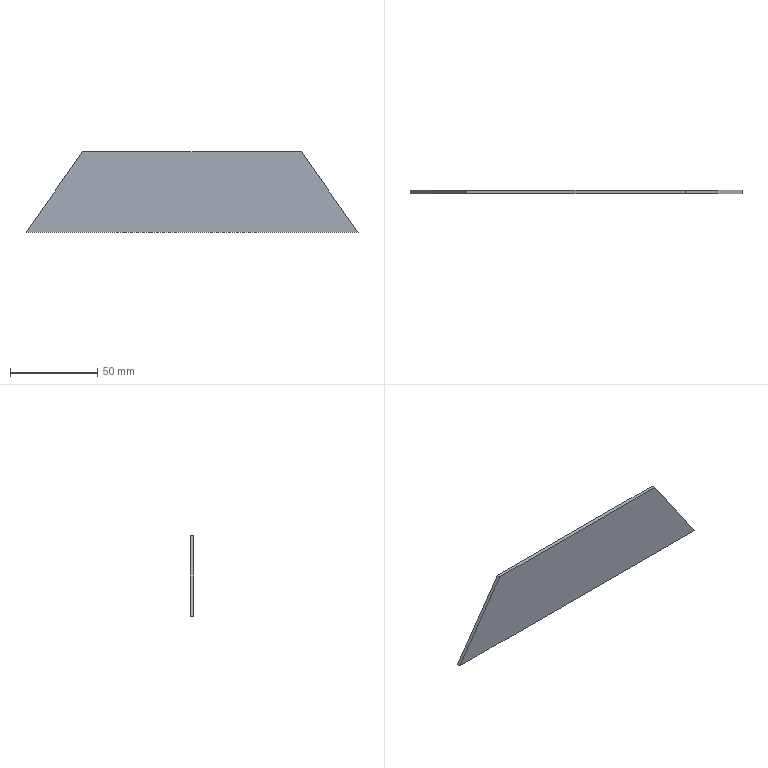Part | SolidWorks | features BaseBody 1 | 1 solid | 6 faces | box 189.769 x 2 x 46.25 mm | volume 14558 mm3 | plane 6
STEP:
#1=CARTESIAN_POINT('',(-157.385,2.,-46.25));
#2=VERTEX_POINT('',#1);
#3=CARTESIAN_POINT('',(-125.,2.,0.));
#4=VERTEX_POINT('',#3);
#5=CARTESIAN_POINT('',(-125.,2.,0.));
#6=DIRECTION('',(0.5736,0.,0.8192));
#7=VECTOR('',#6,1000.);
#8=LINE('',#5,#7);
#9=EDGE_CURVE('',#2,#4,#8,.T.);
#10=ORIENTED_EDGE('',*,*,#9,.T.);
#11=CARTESIAN_POINT('',(0.,2.,0.));
#12=VERTEX_POINT('',#11);
#13=CARTESIAN_POINT('',(0.,2.,0.));
#14=DIRECTION('',(1.,0.,0.));
#15=VECTOR('',#14,1000.);
#16=LINE('',#13,#15);
#17=EDGE_CURVE('',#4,#12,#16,.T.);
#18=ORIENTED_EDGE('',*,*,#17,.T.);
#19=CARTESIAN_POINT('',(32.385,2.,-46.25));
#20=VERTEX_POINT('',#19);
#21=CARTESIAN_POINT('',(0.,2.,0.));
#22=DIRECTION('',(0.5736,0.,-0.8192));
#23=VECTOR('',#22,1000.);
#24=LINE('',#21,#23);
#25=EDGE_CURVE('',#12,#20,#24,.T.);
#26=ORIENTED_EDGE('',*,*,#25,.T.);
#27=CARTESIAN_POINT('',(32.385,2.,-46.25));
#28=DIRECTION('',(-1.,0.,0.));
#29=VECTOR('',#28,1000.);
#30=LINE('',#27,#29);
#31=EDGE_CURVE('',#20,#2,#30,.T.);
#32=ORIENTED_EDGE('',*,*,#31,.T.);
#33=EDGE_LOOP('',(#10,#18,#26,#32));
#34=FACE_OUTER_BOUND('',#33,.T.);
#35=CARTESIAN_POINT('',(0.,2.,0.));
#36=DIRECTION('',(0.,1.,0.));
#37=DIRECTION('',(1.,0.,0.));
#38=AXIS2_PLACEMENT_3D('',#35,#36,#37);
#39=PLANE('',#38);
#40=ADVANCED_FACE('',(#34),#39,.T.);
#41=CARTESIAN_POINT('',(-157.385,0.,-46.25));
#42=VERTEX_POINT('',#41);
#43=CARTESIAN_POINT('',(-157.385,2.,-46.25));
#44=DIRECTION('',(0.,1.,0.));
#45=VECTOR('',#44,1000.);
#46=LINE('',#43,#45);
#47=EDGE_CURVE('',#42,#2,#46,.T.);
#48=ORIENTED_EDGE('',*,*,#47,.T.);
#49=ORIENTED_EDGE('',*,*,#31,.F.);
#50=CARTESIAN_POINT('',(32.385,0.,-46.25));
#51=VERTEX_POINT('',#50);
#52=CARTESIAN_POINT('',(32.385,2.,-46.25));
#53=DIRECTION('',(0.,-1.,0.));
#54=VECTOR('',#53,1000.);
#55=LINE('',#52,#54);
#56=EDGE_CURVE('',#20,#51,#55,.T.);
#57=ORIENTED_EDGE('',*,*,#56,.T.);
#58=CARTESIAN_POINT('',(0.,0.,-46.25));
#59=DIRECTION('',(-1.,0.,0.));
#60=VECTOR('',#59,1000.);
#61=LINE('',#58,#60);
#62=EDGE_CURVE('',#51,#42,#61,.T.);
#63=ORIENTED_EDGE('',*,*,#62,.T.);
#64=EDGE_LOOP('',(#48,#49,#57,#63));
#65=FACE_OUTER_BOUND('',#64,.T.);
#66=CARTESIAN_POINT('',(32.385,2.,-46.25));
#67=DIRECTION('',(0.,0.,1.));
#68=DIRECTION('',(1.,0.,0.));
#69=AXIS2_PLACEMENT_3D('',#66,#67,#68);
#70=PLANE('',#69);
#71=ADVANCED_FACE('',(#65),#70,.F.);
#72=CARTESIAN_POINT('',(-125.,0.,0.));
#73=VERTEX_POINT('',#72);
#74=CARTESIAN_POINT('',(-125.,2.,0.));
#75=DIRECTION('',(0.,1.,0.));
#76=VECTOR('',#75,1000.);
#77=LINE('',#74,#76);
#78=EDGE_CURVE('',#73,#4,#77,.T.);
#79=ORIENTED_EDGE('',*,*,#78,.T.);
#80=ORIENTED_EDGE('',*,*,#9,.F.);
#81=ORIENTED_EDGE('',*,*,#47,.F.);
#82=CARTESIAN_POINT('',(-157.385,0.,-46.25));
#83=DIRECTION('',(0.5736,0.,0.8192));
#84=VECTOR('',#83,1000.);
#85=LINE('',#82,#84);
#86=EDGE_CURVE('',#42,#73,#85,.T.);
#87=ORIENTED_EDGE('',*,*,#86,.T.);
#88=EDGE_LOOP('',(#79,#80,#81,#87));
#89=FACE_OUTER_BOUND('',#88,.T.);
#90=CARTESIAN_POINT('',(-125.,2.,0.));
#91=DIRECTION('',(0.8192,0.,-0.5736));
#92=DIRECTION('',(0.,-1.,0.));
#93=AXIS2_PLACEMENT_3D('',#90,#91,#92);
#94=PLANE('',#93);
#95=ADVANCED_FACE('',(#89),#94,.F.);
#96=CARTESIAN_POINT('',(0.,0.,0.));
#97=VERTEX_POINT('',#96);
#98=CARTESIAN_POINT('',(0.,2.,0.));
#99=DIRECTION('',(0.,1.,0.));
#100=VECTOR('',#99,1000.);
#101=LINE('',#98,#100);
#102=EDGE_CURVE('',#97,#12,#101,.T.);
#103=ORIENTED_EDGE('',*,*,#102,.T.);
#104=ORIENTED_EDGE('',*,*,#17,.F.);
#105=ORIENTED_EDGE('',*,*,#78,.F.);
#106=CARTESIAN_POINT('',(0.,0.,0.));
#107=DIRECTION('',(1.,0.,0.));
#108=VECTOR('',#107,1000.);
#109=LINE('',#106,#108);
#110=EDGE_CURVE('',#73,#97,#109,.T.);
#111=ORIENTED_EDGE('',*,*,#110,.T.);
#112=EDGE_LOOP('',(#103,#104,#105,#111));
#113=FACE_OUTER_BOUND('',#112,.T.);
#114=CARTESIAN_POINT('',(0.,2.,0.));
#115=DIRECTION('',(0.,0.,-1.));
#116=DIRECTION('',(-1.,0.,0.));
#117=AXIS2_PLACEMENT_3D('',#114,#115,#116);
#118=PLANE('',#117);
#119=ADVANCED_FACE('',(#113),#118,.F.);
#120=ORIENTED_EDGE('',*,*,#56,.F.);
#121=ORIENTED_EDGE('',*,*,#25,.F.);
#122=ORIENTED_EDGE('',*,*,#102,.F.);
#123=CARTESIAN_POINT('',(0.,0.,0.));
#124=DIRECTION('',(0.5736,0.,-0.8192));
#125=VECTOR('',#124,1000.);
#126=LINE('',#123,#125);
#127=EDGE_CURVE('',#97,#51,#126,.T.);
#128=ORIENTED_EDGE('',*,*,#127,.T.);
#129=EDGE_LOOP('',(#120,#121,#122,#128));
#130=FACE_OUTER_BOUND('',#129,.T.);
#131=CARTESIAN_POINT('',(0.,2.,0.));
#132=DIRECTION('',(-0.8192,0.,-0.5736));
#133=DIRECTION('',(-0.5736,0.,0.8192));
#134=AXIS2_PLACEMENT_3D('',#131,#132,#133);
#135=PLANE('',#134);
#136=ADVANCED_FACE('',(#130),#135,.F.);
#137=ORIENTED_EDGE('',*,*,#110,.F.);
#138=ORIENTED_EDGE('',*,*,#86,.F.);
#139=ORIENTED_EDGE('',*,*,#62,.F.);
#140=ORIENTED_EDGE('',*,*,#127,.F.);
#141=EDGE_LOOP('',(#137,#138,#139,#140));
#142=FACE_OUTER_BOUND('',#141,.T.);
#143=CARTESIAN_POINT('',(0.,0.,0.));
#144=DIRECTION('',(0.,1.,0.));
#145=DIRECTION('',(1.,0.,0.));
#146=AXIS2_PLACEMENT_3D('',#143,#144,#145);
#147=PLANE('',#146);
#148=ADVANCED_FACE('',(#142),#147,.F.);
#149=CLOSED_SHELL('',(#40,#71,#95,#119,#136,#148));
#150=MANIFOLD_SOLID_BREP('',#149);
#151=CARTESIAN_POINT('',(0.,0.,0.));
#152=DIRECTION('',(0.,0.,1.));
#153=DIRECTION('',(1.,0.,0.));
#154=AXIS2_PLACEMENT_3D('',#151,#152,#153);
#155=(LENGTH_UNIT()NAMED_UNIT(*)SI_UNIT(.MILLI.,.METRE.));
#156=UNCERTAINTY_MEASURE_WITH_UNIT(LENGTH_MEASURE(0.00001),#155,'','');
#157=(NAMED_UNIT(*)PLANE_ANGLE_UNIT()SI_UNIT($,.RADIAN.));
#158=(NAMED_UNIT(*)SI_UNIT($,.STERADIAN.)SOLID_ANGLE_UNIT());
#159=(GEOMETRIC_REPRESENTATION_CONTEXT(3)GLOBAL_UNCERTAINTY_ASSIGNED_CONTEXT((#156))GLOBAL_UNIT_ASSIGNED_CONTEXT((#155,#157,#158))REPRESENTATION_CONTEXT('',''));
#160=ADVANCED_BREP_SHAPE_REPRESENTATION('',(#150,#154),#159);